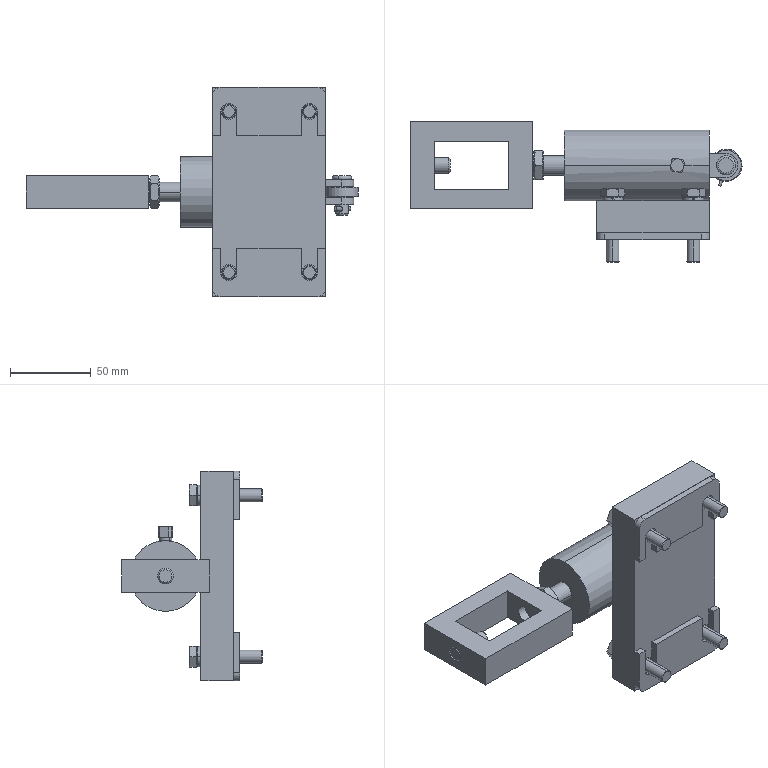Part | SolidWorks | features CompositeCurve 2 | 21 solids | 330 faces | box 206.02 x 86.9 x 130 mm | volume 377637 mm3 | plane 146 | cylinder 103 | cone 61 | torus 18 | spline 2 | commonest cylinder face diameters 10 x20 8 x18 8.68 x12 12.88 x12 9.7 x5 30 x5